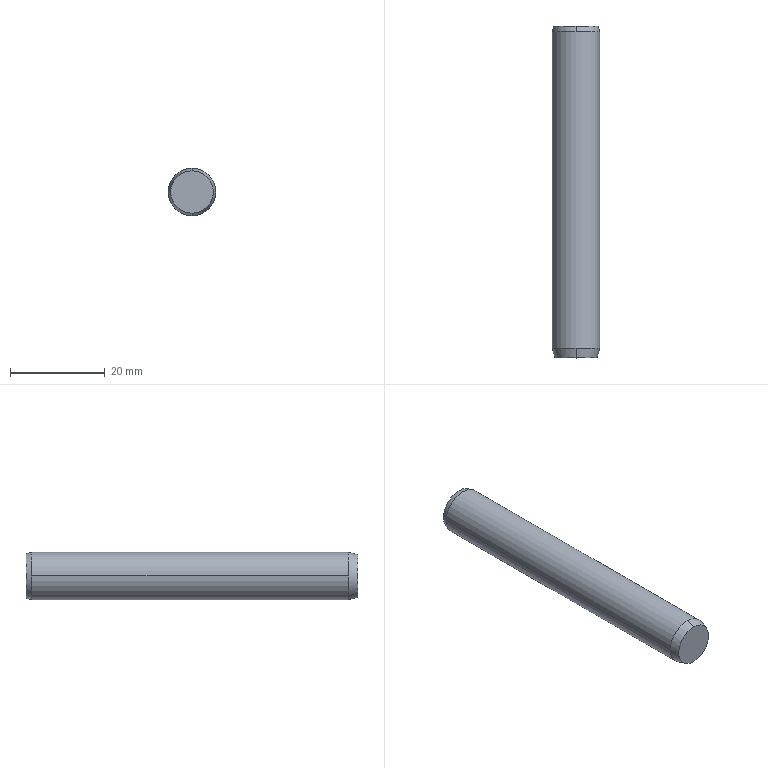Part | STEP file | 1 solid | 16 faces | box 10 x 70 x 10 mm | volume 5144 mm3 | cone 8 | cylinder 6 | plane 2 | commonest cylinder face diameters 4.917 x2 6.4 x2 10 x2
STEP:
#1=CARTESIAN_POINT('',(0.,-70.,4.464));
#2=VERTEX_POINT('',#1);
#3=CARTESIAN_POINT('',(0.,-70.,-4.464));
#4=VERTEX_POINT('',#3);
#5=CARTESIAN_POINT('',(0.,-70.,0.));
#6=DIRECTION('',(0.,1.,0.));
#7=DIRECTION('',(0.,0.,1.));
#8=AXIS2_PLACEMENT_3D('',#5,#6,#7);
#9=CIRCLE('',#8,4.464);
#10=EDGE_CURVE('',#2,#4,#9,.T.);
#11=ORIENTED_EDGE('',*,*,#10,.T.);
#12=CARTESIAN_POINT('',(0.,-68.,-5.));
#13=VERTEX_POINT('',#12);
#14=CARTESIAN_POINT('',(0.,-70.,-4.464));
#15=DIRECTION('',(0.,0.9659,-0.2588));
#16=VECTOR('',#15,1000.);
#17=LINE('',#14,#16);
#18=EDGE_CURVE('',#4,#13,#17,.T.);
#19=ORIENTED_EDGE('',*,*,#18,.T.);
#20=CARTESIAN_POINT('',(5.,-68.,0.));
#21=VERTEX_POINT('',#20);
#22=CARTESIAN_POINT('',(0.,-68.,0.));
#23=DIRECTION('',(0.,1.,0.));
#24=DIRECTION('',(0.,0.,1.));
#25=AXIS2_PLACEMENT_3D('',#22,#23,#24);
#26=CIRCLE('',#25,5.);
#27=EDGE_CURVE('',#21,#13,#26,.T.);
#28=ORIENTED_EDGE('',*,*,#27,.F.);
#29=CARTESIAN_POINT('',(0.,-68.,5.));
#30=VERTEX_POINT('',#29);
#31=CARTESIAN_POINT('',(0.,-68.,0.));
#32=DIRECTION('',(0.,1.,0.));
#33=DIRECTION('',(0.,0.,1.));
#34=AXIS2_PLACEMENT_3D('',#31,#32,#33);
#35=CIRCLE('',#34,5.);
#36=EDGE_CURVE('',#30,#21,#35,.T.);
#37=ORIENTED_EDGE('',*,*,#36,.F.);
#38=CARTESIAN_POINT('',(0.,-70.,4.464));
#39=DIRECTION('',(0.,0.9659,0.2588));
#40=VECTOR('',#39,1000.);
#41=LINE('',#38,#40);
#42=EDGE_CURVE('',#2,#30,#41,.T.);
#43=ORIENTED_EDGE('',*,*,#42,.F.);
#44=EDGE_LOOP('',(#11,#19,#28,#37,#43));
#45=FACE_OUTER_BOUND('',#44,.T.);
#46=CARTESIAN_POINT('',(0.,-70.,0.));
#47=DIRECTION('',(0.,1.,0.));
#48=DIRECTION('',(0.,0.,1.));
#49=AXIS2_PLACEMENT_3D('',#46,#47,#48);
#50=CONICAL_SURFACE('',#49,4.464,0.2618);
#51=ADVANCED_FACE('',(#45),#50,.T.);
#52=CARTESIAN_POINT('',(-5.,-68.,0.));
#53=VERTEX_POINT('',#52);
#54=CARTESIAN_POINT('',(0.,-68.,0.));
#55=DIRECTION('',(0.,1.,0.));
#56=DIRECTION('',(0.,0.,1.));
#57=AXIS2_PLACEMENT_3D('',#54,#55,#56);
#58=CIRCLE('',#57,5.);
#59=EDGE_CURVE('',#53,#30,#58,.T.);
#60=ORIENTED_EDGE('',*,*,#59,.T.);
#61=ORIENTED_EDGE('',*,*,#36,.T.);
#62=CARTESIAN_POINT('',(5.,-1.2,0.));
#63=VERTEX_POINT('',#62);
#64=CARTESIAN_POINT('',(5.,-17.42,0.));
#65=DIRECTION('',(0.,1.,0.));
#66=VECTOR('',#65,1000.);
#67=LINE('',#64,#66);
#68=EDGE_CURVE('',#21,#63,#67,.T.);
#69=ORIENTED_EDGE('',*,*,#68,.T.);
#70=CARTESIAN_POINT('',(0.,-1.2,5.));
#71=VERTEX_POINT('',#70);
#72=CARTESIAN_POINT('',(0.,-1.2,0.));
#73=DIRECTION('',(0.,1.,0.));
#74=DIRECTION('',(0.,0.,1.));
#75=AXIS2_PLACEMENT_3D('',#72,#73,#74);
#76=CIRCLE('',#75,5.);
#77=EDGE_CURVE('',#71,#63,#76,.T.);
#78=ORIENTED_EDGE('',*,*,#77,.F.);
#79=CARTESIAN_POINT('',(-5.,-1.2,0.));
#80=VERTEX_POINT('',#79);
#81=CARTESIAN_POINT('',(0.,-1.2,0.));
#82=DIRECTION('',(0.,1.,0.));
#83=DIRECTION('',(0.,0.,1.));
#84=AXIS2_PLACEMENT_3D('',#81,#82,#83);
#85=CIRCLE('',#84,5.);
#86=EDGE_CURVE('',#80,#71,#85,.T.);
#87=ORIENTED_EDGE('',*,*,#86,.F.);
#88=CARTESIAN_POINT('',(-5.,-17.42,0.));
#89=DIRECTION('',(0.,1.,0.));
#90=VECTOR('',#89,1000.);
#91=LINE('',#88,#90);
#92=EDGE_CURVE('',#53,#80,#91,.T.);
#93=ORIENTED_EDGE('',*,*,#92,.F.);
#94=EDGE_LOOP('',(#60,#61,#69,#78,#87,#93));
#95=FACE_OUTER_BOUND('',#94,.T.);
#96=CARTESIAN_POINT('',(0.,-17.42,0.));
#97=DIRECTION('',(0.,1.,0.));
#98=DIRECTION('',(-1.,0.,0.));
#99=AXIS2_PLACEMENT_3D('',#96,#97,#98);
#100=CYLINDRICAL_SURFACE('',#99,5.);
#101=ADVANCED_FACE('',(#95),#100,.T.);
#102=CARTESIAN_POINT('',(0.,0.,4.678));
#103=VERTEX_POINT('',#102);
#104=CARTESIAN_POINT('',(0.,0.,-4.678));
#105=VERTEX_POINT('',#104);
#106=CARTESIAN_POINT('',(0.,0.,0.));
#107=DIRECTION('',(0.,1.,0.));
#108=DIRECTION('',(0.,0.,1.));
#109=AXIS2_PLACEMENT_3D('',#106,#107,#108);
#110=CIRCLE('',#109,4.678);
#111=EDGE_CURVE('',#103,#105,#110,.T.);
#112=ORIENTED_EDGE('',*,*,#111,.F.);
#113=CARTESIAN_POINT('',(0.,-1.2,5.));
#114=DIRECTION('',(0.,-0.9659,0.2588));
#115=VECTOR('',#114,1000.);
#116=LINE('',#113,#115);
#117=EDGE_CURVE('',#103,#71,#116,.T.);
#118=ORIENTED_EDGE('',*,*,#117,.T.);
#119=ORIENTED_EDGE('',*,*,#77,.T.);
#120=CARTESIAN_POINT('',(0.,-1.2,-5.));
#121=VERTEX_POINT('',#120);
#122=CARTESIAN_POINT('',(0.,-1.2,0.));
#123=DIRECTION('',(0.,1.,0.));
#124=DIRECTION('',(0.,0.,1.));
#125=AXIS2_PLACEMENT_3D('',#122,#123,#124);
#126=CIRCLE('',#125,5.);
#127=EDGE_CURVE('',#63,#121,#126,.T.);
#128=ORIENTED_EDGE('',*,*,#127,.T.);
#129=CARTESIAN_POINT('',(0.,-1.2,-5.));
#130=DIRECTION('',(0.,-0.9659,-0.2588));
#131=VECTOR('',#130,1000.);
#132=LINE('',#129,#131);
#133=EDGE_CURVE('',#105,#121,#132,.T.);
#134=ORIENTED_EDGE('',*,*,#133,.F.);
#135=EDGE_LOOP('',(#112,#118,#119,#128,#134));
#136=FACE_OUTER_BOUND('',#135,.T.);
#137=CARTESIAN_POINT('',(0.,-1.2,0.));
#138=DIRECTION('',(0.,-1.,0.));
#139=DIRECTION('',(0.,0.,-1.));
#140=AXIS2_PLACEMENT_3D('',#137,#138,#139);
#141=CONICAL_SURFACE('',#140,5.,0.2618);
#142=ADVANCED_FACE('',(#136),#141,.T.);
#143=CARTESIAN_POINT('',(0.,-17.42,0.));
#144=VERTEX_POINT('',#143);
#145=CARTESIAN_POINT('',(-2.459,-16.,0.));
#146=VERTEX_POINT('',#145);
#147=CARTESIAN_POINT('',(-2.459,-16.,0.));
#148=DIRECTION('',(-0.866,0.5,0.));
#149=VECTOR('',#148,1000.);
#150=LINE('',#147,#149);
#151=EDGE_CURVE('',#144,#146,#150,.T.);
#152=ORIENTED_EDGE('',*,*,#151,.F.);
#153=CARTESIAN_POINT('',(2.459,-16.,0.));
#154=VERTEX_POINT('',#153);
#155=CARTESIAN_POINT('',(2.459,-16.,0.));
#156=DIRECTION('',(0.866,0.5,0.));
#157=VECTOR('',#156,1000.);
#158=LINE('',#155,#157);
#159=EDGE_CURVE('',#144,#154,#158,.T.);
#160=ORIENTED_EDGE('',*,*,#159,.T.);
#161=CARTESIAN_POINT('',(0.,-16.,0.));
#162=DIRECTION('',(0.,1.,0.));
#163=DIRECTION('',(-1.,0.,0.));
#164=AXIS2_PLACEMENT_3D('',#161,#162,#163);
#165=CIRCLE('',#164,2.459);
#166=EDGE_CURVE('',#154,#146,#165,.T.);
#167=ORIENTED_EDGE('',*,*,#166,.T.);
#168=EDGE_LOOP('',(#152,#160,#167));
#169=FACE_OUTER_BOUND('',#168,.T.);
#170=CARTESIAN_POINT('',(0.,-16.,0.));
#171=DIRECTION('',(0.,1.,0.));
#172=DIRECTION('',(-1.,0.,0.));
#173=AXIS2_PLACEMENT_3D('',#170,#171,#172);
#174=CONICAL_SURFACE('',#173,2.459,1.047);
#175=ADVANCED_FACE('',(#169),#174,.F.);
#176=ORIENTED_EDGE('',*,*,#166,.F.);
#177=CARTESIAN_POINT('',(2.459,-1.628,0.));
#178=VERTEX_POINT('',#177);
#179=CARTESIAN_POINT('',(2.459,-17.42,0.));
#180=DIRECTION('',(0.,1.,0.));
#181=VECTOR('',#180,1000.);
#182=LINE('',#179,#181);
#183=EDGE_CURVE('',#154,#178,#182,.T.);
#184=ORIENTED_EDGE('',*,*,#183,.T.);
#185=CARTESIAN_POINT('',(-2.459,-1.628,0.));
#186=VERTEX_POINT('',#185);
#187=CARTESIAN_POINT('',(0.,-1.628,0.));
#188=DIRECTION('',(0.,1.,0.));
#189=DIRECTION('',(-1.,0.,0.));
#190=AXIS2_PLACEMENT_3D('',#187,#188,#189);
#191=CIRCLE('',#190,2.459);
#192=EDGE_CURVE('',#178,#186,#191,.T.);
#193=ORIENTED_EDGE('',*,*,#192,.T.);
#194=CARTESIAN_POINT('',(-2.459,-17.42,0.));
#195=DIRECTION('',(0.,1.,0.));
#196=VECTOR('',#195,1000.);
#197=LINE('',#194,#196);
#198=EDGE_CURVE('',#146,#186,#197,.T.);
#199=ORIENTED_EDGE('',*,*,#198,.F.);
#200=EDGE_LOOP('',(#176,#184,#193,#199));
#201=FACE_OUTER_BOUND('',#200,.T.);
#202=CARTESIAN_POINT('',(0.,-17.42,0.));
#203=DIRECTION('',(0.,1.,0.));
#204=DIRECTION('',(-1.,0.,0.));
#205=AXIS2_PLACEMENT_3D('',#202,#203,#204);
#206=CYLINDRICAL_SURFACE('',#205,2.459);
#207=ADVANCED_FACE('',(#201),#206,.F.);
#208=ORIENTED_EDGE('',*,*,#192,.F.);
#209=CARTESIAN_POINT('',(3.2,-1.2,0.));
#210=VERTEX_POINT('',#209);
#211=CARTESIAN_POINT('',(3.2,-1.2,0.));
#212=DIRECTION('',(0.866,0.5,0.));
#213=VECTOR('',#212,1000.);
#214=LINE('',#211,#213);
#215=EDGE_CURVE('',#178,#210,#214,.T.);
#216=ORIENTED_EDGE('',*,*,#215,.T.);
#217=CARTESIAN_POINT('',(-3.2,-1.2,0.));
#218=VERTEX_POINT('',#217);
#219=CARTESIAN_POINT('',(0.,-1.2,0.));
#220=DIRECTION('',(0.,1.,0.));
#221=DIRECTION('',(-1.,0.,0.));
#222=AXIS2_PLACEMENT_3D('',#219,#220,#221);
#223=CIRCLE('',#222,3.2);
#224=EDGE_CURVE('',#210,#218,#223,.T.);
#225=ORIENTED_EDGE('',*,*,#224,.T.);
#226=CARTESIAN_POINT('',(-3.2,-1.2,0.));
#227=DIRECTION('',(-0.866,0.5,0.));
#228=VECTOR('',#227,1000.);
#229=LINE('',#226,#228);
#230=EDGE_CURVE('',#186,#218,#229,.T.);
#231=ORIENTED_EDGE('',*,*,#230,.F.);
#232=EDGE_LOOP('',(#208,#216,#225,#231));
#233=FACE_OUTER_BOUND('',#232,.T.);
#234=CARTESIAN_POINT('',(0.,-1.2,0.));
#235=DIRECTION('',(0.,1.,0.));
#236=DIRECTION('',(-1.,0.,0.));
#237=AXIS2_PLACEMENT_3D('',#234,#235,#236);
#238=CONICAL_SURFACE('',#237,3.2,1.047);
#239=ADVANCED_FACE('',(#233),#238,.F.);
#240=ORIENTED_EDGE('',*,*,#224,.F.);
#241=CARTESIAN_POINT('',(3.2,0.,0.));
#242=VERTEX_POINT('',#241);
#243=CARTESIAN_POINT('',(3.2,-17.42,0.));
#244=DIRECTION('',(0.,1.,0.));
#245=VECTOR('',#244,1000.);
#246=LINE('',#243,#245);
#247=EDGE_CURVE('',#210,#242,#246,.T.);
#248=ORIENTED_EDGE('',*,*,#247,.T.);
#249=CARTESIAN_POINT('',(-3.2,0.,0.));
#250=VERTEX_POINT('',#249);
#251=CARTESIAN_POINT('',(0.,0.,0.));
#252=DIRECTION('',(0.,1.,0.));
#253=DIRECTION('',(-1.,0.,0.));
#254=AXIS2_PLACEMENT_3D('',#251,#252,#253);
#255=CIRCLE('',#254,3.2);
#256=EDGE_CURVE('',#242,#250,#255,.T.);
#257=ORIENTED_EDGE('',*,*,#256,.T.);
#258=CARTESIAN_POINT('',(-3.2,-17.42,0.));
#259=DIRECTION('',(0.,1.,0.));
#260=VECTOR('',#259,1000.);
#261=LINE('',#258,#260);
#262=EDGE_CURVE('',#218,#250,#261,.T.);
#263=ORIENTED_EDGE('',*,*,#262,.F.);
#264=EDGE_LOOP('',(#240,#248,#257,#263));
#265=FACE_OUTER_BOUND('',#264,.T.);
#266=CARTESIAN_POINT('',(0.,-17.42,0.));
#267=DIRECTION('',(0.,1.,0.));
#268=DIRECTION('',(-1.,0.,0.));
#269=AXIS2_PLACEMENT_3D('',#266,#267,#268);
#270=CYLINDRICAL_SURFACE('',#269,3.2);
#271=ADVANCED_FACE('',(#265),#270,.F.);
#272=CARTESIAN_POINT('',(0.,0.,0.));
#273=DIRECTION('',(0.,1.,0.));
#274=DIRECTION('',(-1.,0.,0.));
#275=AXIS2_PLACEMENT_3D('',#272,#273,#274);
#276=CIRCLE('',#275,3.2);
#277=EDGE_CURVE('',#250,#242,#276,.T.);
#278=ORIENTED_EDGE('',*,*,#277,.F.);
#279=ORIENTED_EDGE('',*,*,#256,.F.);
#280=EDGE_LOOP('',(#278,#279));
#281=FACE_BOUND('',#280,.T.);
#282=CARTESIAN_POINT('',(0.,0.,0.));
#283=DIRECTION('',(0.,1.,0.));
#284=DIRECTION('',(0.,0.,1.));
#285=AXIS2_PLACEMENT_3D('',#282,#283,#284);
#286=CIRCLE('',#285,4.678);
#287=EDGE_CURVE('',#105,#103,#286,.T.);
#288=ORIENTED_EDGE('',*,*,#287,.T.);
#289=ORIENTED_EDGE('',*,*,#111,.T.);
#290=EDGE_LOOP('',(#288,#289));
#291=FACE_OUTER_BOUND('',#290,.T.);
#292=CARTESIAN_POINT('',(5.,0.,0.));
#293=DIRECTION('',(0.,-1.,0.));
#294=DIRECTION('',(1.,0.,0.));
#295=AXIS2_PLACEMENT_3D('',#292,#293,#294);
#296=PLANE('',#295);
#297=ADVANCED_FACE('',(#281,#291),#296,.F.);
#298=ORIENTED_EDGE('',*,*,#247,.F.);
#299=CARTESIAN_POINT('',(0.,-1.2,0.));
#300=DIRECTION('',(0.,1.,0.));
#301=DIRECTION('',(-1.,0.,0.));
#302=AXIS2_PLACEMENT_3D('',#299,#300,#301);
#303=CIRCLE('',#302,3.2);
#304=EDGE_CURVE('',#218,#210,#303,.T.);
#305=ORIENTED_EDGE('',*,*,#304,.F.);
#306=ORIENTED_EDGE('',*,*,#262,.T.);
#307=ORIENTED_EDGE('',*,*,#277,.T.);
#308=EDGE_LOOP('',(#298,#305,#306,#307));
#309=FACE_OUTER_BOUND('',#308,.T.);
#310=CARTESIAN_POINT('',(0.,-17.42,0.));
#311=DIRECTION('',(0.,1.,0.));
#312=DIRECTION('',(-1.,0.,0.));
#313=AXIS2_PLACEMENT_3D('',#310,#311,#312);
#314=CYLINDRICAL_SURFACE('',#313,3.2);
#315=ADVANCED_FACE('',(#309),#314,.F.);
#316=ORIENTED_EDGE('',*,*,#215,.F.);
#317=CARTESIAN_POINT('',(0.,-1.628,0.));
#318=DIRECTION('',(0.,1.,0.));
#319=DIRECTION('',(-1.,0.,0.));
#320=AXIS2_PLACEMENT_3D('',#317,#318,#319);
#321=CIRCLE('',#320,2.459);
#322=EDGE_CURVE('',#186,#178,#321,.T.);
#323=ORIENTED_EDGE('',*,*,#322,.F.);
#324=ORIENTED_EDGE('',*,*,#230,.T.);
#325=ORIENTED_EDGE('',*,*,#304,.T.);
#326=EDGE_LOOP('',(#316,#323,#324,#325));
#327=FACE_OUTER_BOUND('',#326,.T.);
#328=CARTESIAN_POINT('',(0.,-1.2,0.));
#329=DIRECTION('',(0.,1.,0.));
#330=DIRECTION('',(-1.,0.,0.));
#331=AXIS2_PLACEMENT_3D('',#328,#329,#330);
#332=CONICAL_SURFACE('',#331,3.2,1.047);
#333=ADVANCED_FACE('',(#327),#332,.F.);
#334=ORIENTED_EDGE('',*,*,#183,.F.);
#335=CARTESIAN_POINT('',(0.,-16.,0.));
#336=DIRECTION('',(0.,1.,0.));
#337=DIRECTION('',(-1.,0.,0.));
#338=AXIS2_PLACEMENT_3D('',#335,#336,#337);
#339=CIRCLE('',#338,2.459);
#340=EDGE_CURVE('',#146,#154,#339,.T.);
#341=ORIENTED_EDGE('',*,*,#340,.F.);
#342=ORIENTED_EDGE('',*,*,#198,.T.);
#343=ORIENTED_EDGE('',*,*,#322,.T.);
#344=EDGE_LOOP('',(#334,#341,#342,#343));
#345=FACE_OUTER_BOUND('',#344,.T.);
#346=CARTESIAN_POINT('',(0.,-17.42,0.));
#347=DIRECTION('',(0.,1.,0.));
#348=DIRECTION('',(-1.,0.,0.));
#349=AXIS2_PLACEMENT_3D('',#346,#347,#348);
#350=CYLINDRICAL_SURFACE('',#349,2.459);
#351=ADVANCED_FACE('',(#345),#350,.F.);
#352=ORIENTED_EDGE('',*,*,#159,.F.);
#353=ORIENTED_EDGE('',*,*,#151,.T.);
#354=ORIENTED_EDGE('',*,*,#340,.T.);
#355=EDGE_LOOP('',(#352,#353,#354));
#356=FACE_OUTER_BOUND('',#355,.T.);
#357=CARTESIAN_POINT('',(0.,-16.,0.));
#358=DIRECTION('',(0.,1.,0.));
#359=DIRECTION('',(-1.,0.,0.));
#360=AXIS2_PLACEMENT_3D('',#357,#358,#359);
#361=CONICAL_SURFACE('',#360,2.459,1.047);
#362=ADVANCED_FACE('',(#356),#361,.F.);
#363=ORIENTED_EDGE('',*,*,#117,.F.);
#364=ORIENTED_EDGE('',*,*,#287,.F.);
#365=ORIENTED_EDGE('',*,*,#133,.T.);
#366=CARTESIAN_POINT('',(0.,-1.2,0.));
#367=DIRECTION('',(0.,1.,0.));
#368=DIRECTION('',(0.,0.,1.));
#369=AXIS2_PLACEMENT_3D('',#366,#367,#368);
#370=CIRCLE('',#369,5.);
#371=EDGE_CURVE('',#121,#80,#370,.T.);
#372=ORIENTED_EDGE('',*,*,#371,.T.);
#373=ORIENTED_EDGE('',*,*,#86,.T.);
#374=EDGE_LOOP('',(#363,#364,#365,#372,#373));
#375=FACE_OUTER_BOUND('',#374,.T.);
#376=CARTESIAN_POINT('',(0.,-1.2,0.));
#377=DIRECTION('',(0.,-1.,0.));
#378=DIRECTION('',(0.,0.,-1.));
#379=AXIS2_PLACEMENT_3D('',#376,#377,#378);
#380=CONICAL_SURFACE('',#379,5.,0.2618);
#381=ADVANCED_FACE('',(#375),#380,.T.);
#382=ORIENTED_EDGE('',*,*,#68,.F.);
#383=ORIENTED_EDGE('',*,*,#27,.T.);
#384=CARTESIAN_POINT('',(0.,-68.,0.));
#385=DIRECTION('',(0.,1.,0.));
#386=DIRECTION('',(0.,0.,1.));
#387=AXIS2_PLACEMENT_3D('',#384,#385,#386);
#388=CIRCLE('',#387,5.);
#389=EDGE_CURVE('',#13,#53,#388,.T.);
#390=ORIENTED_EDGE('',*,*,#389,.T.);
#391=ORIENTED_EDGE('',*,*,#92,.T.);
#392=ORIENTED_EDGE('',*,*,#371,.F.);
#393=ORIENTED_EDGE('',*,*,#127,.F.);
#394=EDGE_LOOP('',(#382,#383,#390,#391,#392,#393));
#395=FACE_OUTER_BOUND('',#394,.T.);
#396=CARTESIAN_POINT('',(0.,-17.42,0.));
#397=DIRECTION('',(0.,1.,0.));
#398=DIRECTION('',(-1.,0.,0.));
#399=AXIS2_PLACEMENT_3D('',#396,#397,#398);
#400=CYLINDRICAL_SURFACE('',#399,5.);
#401=ADVANCED_FACE('',(#395),#400,.T.);
#402=ORIENTED_EDGE('',*,*,#18,.F.);
#403=CARTESIAN_POINT('',(0.,-70.,0.));
#404=DIRECTION('',(0.,1.,0.));
#405=DIRECTION('',(0.,0.,1.));
#406=AXIS2_PLACEMENT_3D('',#403,#404,#405);
#407=CIRCLE('',#406,4.464);
#408=EDGE_CURVE('',#4,#2,#407,.T.);
#409=ORIENTED_EDGE('',*,*,#408,.T.);
#410=ORIENTED_EDGE('',*,*,#42,.T.);
#411=ORIENTED_EDGE('',*,*,#59,.F.);
#412=ORIENTED_EDGE('',*,*,#389,.F.);
#413=EDGE_LOOP('',(#402,#409,#410,#411,#412));
#414=FACE_OUTER_BOUND('',#413,.T.);
#415=CARTESIAN_POINT('',(0.,-70.,0.));
#416=DIRECTION('',(0.,1.,0.));
#417=DIRECTION('',(0.,0.,1.));
#418=AXIS2_PLACEMENT_3D('',#415,#416,#417);
#419=CONICAL_SURFACE('',#418,4.464,0.2618);
#420=ADVANCED_FACE('',(#414),#419,.T.);
#421=ORIENTED_EDGE('',*,*,#10,.F.);
#422=ORIENTED_EDGE('',*,*,#408,.F.);
#423=EDGE_LOOP('',(#421,#422));
#424=FACE_OUTER_BOUND('',#423,.T.);
#425=CARTESIAN_POINT('',(0.,-70.,0.));
#426=DIRECTION('',(0.,1.,0.));
#427=DIRECTION('',(-1.,0.,0.));
#428=AXIS2_PLACEMENT_3D('',#425,#426,#427);
#429=PLANE('',#428);
#430=ADVANCED_FACE('',(#424),#429,.F.);
#431=CLOSED_SHELL('',(#51,#101,#142,#175,#207,#239,#271,#297,#315,#333,#351,#362,#381,#401,#420,#430));
#432=MANIFOLD_SOLID_BREP('',#431);
#433=CARTESIAN_POINT('',(0.,0.,0.));
#434=DIRECTION('',(0.,0.,1.));
#435=DIRECTION('',(1.,0.,0.));
#436=AXIS2_PLACEMENT_3D('',#433,#434,#435);
#437=(LENGTH_UNIT()NAMED_UNIT(*)SI_UNIT(.MILLI.,.METRE.));
#438=UNCERTAINTY_MEASURE_WITH_UNIT(LENGTH_MEASURE(0.00001),#437,'','');
#439=(NAMED_UNIT(*)PLANE_ANGLE_UNIT()SI_UNIT($,.RADIAN.));
#440=(NAMED_UNIT(*)SI_UNIT($,.STERADIAN.)SOLID_ANGLE_UNIT());
#441=(GEOMETRIC_REPRESENTATION_CONTEXT(3)GLOBAL_UNCERTAINTY_ASSIGNED_CONTEXT((#438))GLOBAL_UNIT_ASSIGNED_CONTEXT((#437,#439,#440))REPRESENTATION_CONTEXT('',''));
#442=ADVANCED_BREP_SHAPE_REPRESENTATION('',(#432,#436),#441);